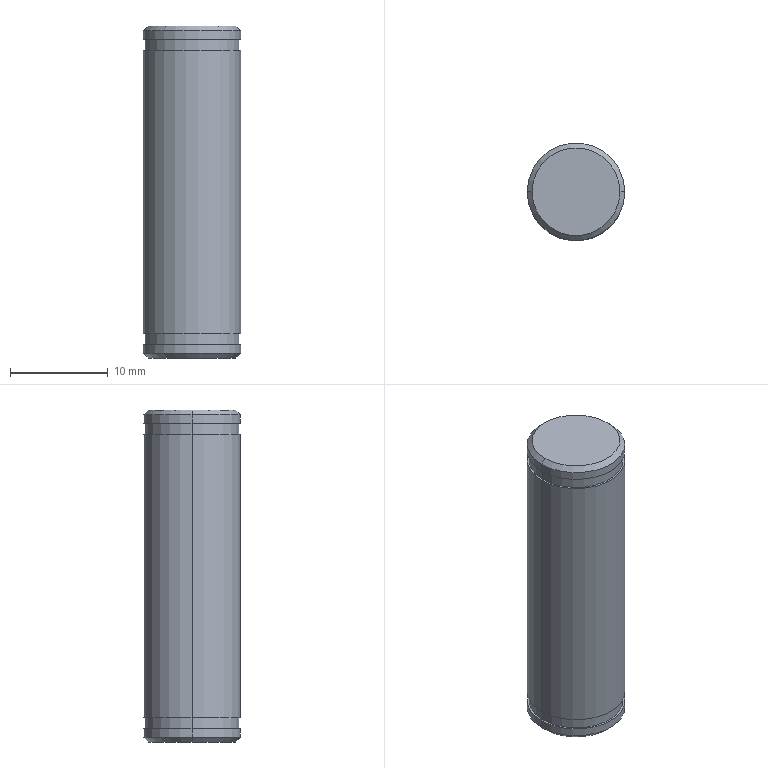Part | STEP file | CD_S03_CD-S03 | 1 solid | 20 faces | box 10 x 10 x 34 mm | volume 2649 mm3 | cylinder 10 | plane 6 | cone 4 | commonest cylinder face diameters 10 x6 9.6 x4
STEP:
#1=CARTESIAN_POINT('',(4.5,0.,-34.));
#2=VERTEX_POINT('',#1);
#3=CARTESIAN_POINT('',(-4.5,0.,-34.));
#4=VERTEX_POINT('',#3);
#5=CARTESIAN_POINT('',(0.,0.,-34.));
#6=DIRECTION('',(0.,0.,1.));
#7=DIRECTION('',(1.,0.,0.));
#8=AXIS2_PLACEMENT_3D('',#5,#6,#7);
#9=CIRCLE('',#8,4.5);
#10=EDGE_CURVE('',#2,#4,#9,.T.);
#11=ORIENTED_EDGE('',*,*,#10,.T.);
#12=CARTESIAN_POINT('',(-5.,0.,-33.5));
#13=VERTEX_POINT('',#12);
#14=CARTESIAN_POINT('',(-4.5,0.,-34.));
#15=DIRECTION('',(-0.7071,0.,0.7071));
#16=VECTOR('',#15,1000.);
#17=LINE('',#14,#16);
#18=EDGE_CURVE('',#4,#13,#17,.T.);
#19=ORIENTED_EDGE('',*,*,#18,.T.);
#20=CARTESIAN_POINT('',(5.,0.,-33.5));
#21=VERTEX_POINT('',#20);
#22=CARTESIAN_POINT('',(0.,0.,-33.5));
#23=DIRECTION('',(0.,0.,1.));
#24=DIRECTION('',(1.,0.,0.));
#25=AXIS2_PLACEMENT_3D('',#22,#23,#24);
#26=CIRCLE('',#25,5.);
#27=EDGE_CURVE('',#21,#13,#26,.T.);
#28=ORIENTED_EDGE('',*,*,#27,.F.);
#29=CARTESIAN_POINT('',(4.5,0.,-34.));
#30=DIRECTION('',(0.7071,0.,0.7071));
#31=VECTOR('',#30,1000.);
#32=LINE('',#29,#31);
#33=EDGE_CURVE('',#2,#21,#32,.T.);
#34=ORIENTED_EDGE('',*,*,#33,.F.);
#35=EDGE_LOOP('',(#11,#19,#28,#34));
#36=FACE_OUTER_BOUND('',#35,.T.);
#37=CARTESIAN_POINT('',(0.,0.,-34.));
#38=DIRECTION('',(0.,0.,1.));
#39=DIRECTION('',(1.,0.,0.));
#40=AXIS2_PLACEMENT_3D('',#37,#38,#39);
#41=CONICAL_SURFACE('',#40,4.5,0.7854);
#42=ADVANCED_FACE('',(#36),#41,.T.);
#43=ORIENTED_EDGE('',*,*,#27,.T.);
#44=CARTESIAN_POINT('',(-5.,0.,-32.65));
#45=VERTEX_POINT('',#44);
#46=CARTESIAN_POINT('',(-5.,0.,-34.));
#47=DIRECTION('',(0.,0.,1.));
#48=VECTOR('',#47,1000.);
#49=LINE('',#46,#48);
#50=EDGE_CURVE('',#13,#45,#49,.T.);
#51=ORIENTED_EDGE('',*,*,#50,.T.);
#52=CARTESIAN_POINT('',(5.,0.,-32.65));
#53=VERTEX_POINT('',#52);
#54=CARTESIAN_POINT('',(0.,0.,-32.65));
#55=DIRECTION('',(0.,0.,1.));
#56=DIRECTION('',(1.,0.,0.));
#57=AXIS2_PLACEMENT_3D('',#54,#55,#56);
#58=CIRCLE('',#57,5.);
#59=EDGE_CURVE('',#53,#45,#58,.T.);
#60=ORIENTED_EDGE('',*,*,#59,.F.);
#61=CARTESIAN_POINT('',(5.,0.,-34.));
#62=DIRECTION('',(0.,0.,1.));
#63=VECTOR('',#62,1000.);
#64=LINE('',#61,#63);
#65=EDGE_CURVE('',#21,#53,#64,.T.);
#66=ORIENTED_EDGE('',*,*,#65,.F.);
#67=EDGE_LOOP('',(#43,#51,#60,#66));
#68=FACE_OUTER_BOUND('',#67,.T.);
#69=CARTESIAN_POINT('',(0.,0.,-34.));
#70=DIRECTION('',(0.,0.,1.));
#71=DIRECTION('',(1.,0.,0.));
#72=AXIS2_PLACEMENT_3D('',#69,#70,#71);
#73=CYLINDRICAL_SURFACE('',#72,5.);
#74=ADVANCED_FACE('',(#68),#73,.T.);
#75=CARTESIAN_POINT('',(4.8,0.,-32.65));
#76=VERTEX_POINT('',#75);
#77=CARTESIAN_POINT('',(-4.8,0.,-32.65));
#78=VERTEX_POINT('',#77);
#79=CARTESIAN_POINT('',(0.,0.,-32.65));
#80=DIRECTION('',(0.,0.,1.));
#81=DIRECTION('',(1.,0.,0.));
#82=AXIS2_PLACEMENT_3D('',#79,#80,#81);
#83=CIRCLE('',#82,4.8);
#84=EDGE_CURVE('',#76,#78,#83,.T.);
#85=ORIENTED_EDGE('',*,*,#84,.T.);
#86=CARTESIAN_POINT('',(-4.8,0.,-31.5));
#87=VERTEX_POINT('',#86);
#88=CARTESIAN_POINT('',(-4.8,0.,-34.));
#89=DIRECTION('',(0.,0.,1.));
#90=VECTOR('',#89,1000.);
#91=LINE('',#88,#90);
#92=EDGE_CURVE('',#78,#87,#91,.T.);
#93=ORIENTED_EDGE('',*,*,#92,.T.);
#94=CARTESIAN_POINT('',(4.8,0.,-31.5));
#95=VERTEX_POINT('',#94);
#96=CARTESIAN_POINT('',(0.,0.,-31.5));
#97=DIRECTION('',(0.,0.,1.));
#98=DIRECTION('',(1.,0.,0.));
#99=AXIS2_PLACEMENT_3D('',#96,#97,#98);
#100=CIRCLE('',#99,4.8);
#101=EDGE_CURVE('',#95,#87,#100,.T.);
#102=ORIENTED_EDGE('',*,*,#101,.F.);
#103=CARTESIAN_POINT('',(4.8,0.,-34.));
#104=DIRECTION('',(0.,0.,1.));
#105=VECTOR('',#104,1000.);
#106=LINE('',#103,#105);
#107=EDGE_CURVE('',#76,#95,#106,.T.);
#108=ORIENTED_EDGE('',*,*,#107,.F.);
#109=EDGE_LOOP('',(#85,#93,#102,#108));
#110=FACE_OUTER_BOUND('',#109,.T.);
#111=CARTESIAN_POINT('',(0.,0.,-34.));
#112=DIRECTION('',(0.,0.,1.));
#113=DIRECTION('',(1.,0.,0.));
#114=AXIS2_PLACEMENT_3D('',#111,#112,#113);
#115=CYLINDRICAL_SURFACE('',#114,4.8);
#116=ADVANCED_FACE('',(#110),#115,.T.);
#117=CARTESIAN_POINT('',(5.,0.,-31.5));
#118=VERTEX_POINT('',#117);
#119=CARTESIAN_POINT('',(-5.,0.,-31.5));
#120=VERTEX_POINT('',#119);
#121=CARTESIAN_POINT('',(0.,0.,-31.5));
#122=DIRECTION('',(0.,0.,1.));
#123=DIRECTION('',(1.,0.,0.));
#124=AXIS2_PLACEMENT_3D('',#121,#122,#123);
#125=CIRCLE('',#124,5.);
#126=EDGE_CURVE('',#118,#120,#125,.T.);
#127=ORIENTED_EDGE('',*,*,#126,.T.);
#128=CARTESIAN_POINT('',(-5.,0.,-2.5));
#129=VERTEX_POINT('',#128);
#130=CARTESIAN_POINT('',(-5.,0.,-34.));
#131=DIRECTION('',(0.,0.,1.));
#132=VECTOR('',#131,1000.);
#133=LINE('',#130,#132);
#134=EDGE_CURVE('',#120,#129,#133,.T.);
#135=ORIENTED_EDGE('',*,*,#134,.T.);
#136=CARTESIAN_POINT('',(5.,0.,-2.5));
#137=VERTEX_POINT('',#136);
#138=CARTESIAN_POINT('',(0.,0.,-2.5));
#139=DIRECTION('',(0.,0.,1.));
#140=DIRECTION('',(1.,0.,0.));
#141=AXIS2_PLACEMENT_3D('',#138,#139,#140);
#142=CIRCLE('',#141,5.);
#143=EDGE_CURVE('',#137,#129,#142,.T.);
#144=ORIENTED_EDGE('',*,*,#143,.F.);
#145=CARTESIAN_POINT('',(5.,0.,-34.));
#146=DIRECTION('',(0.,0.,1.));
#147=VECTOR('',#146,1000.);
#148=LINE('',#145,#147);
#149=EDGE_CURVE('',#118,#137,#148,.T.);
#150=ORIENTED_EDGE('',*,*,#149,.F.);
#151=EDGE_LOOP('',(#127,#135,#144,#150));
#152=FACE_OUTER_BOUND('',#151,.T.);
#153=CARTESIAN_POINT('',(0.,0.,-34.));
#154=DIRECTION('',(0.,0.,1.));
#155=DIRECTION('',(1.,0.,0.));
#156=AXIS2_PLACEMENT_3D('',#153,#154,#155);
#157=CYLINDRICAL_SURFACE('',#156,5.);
#158=ADVANCED_FACE('',(#152),#157,.T.);
#159=CARTESIAN_POINT('',(4.8,0.,-2.5));
#160=VERTEX_POINT('',#159);
#161=CARTESIAN_POINT('',(-4.8,0.,-2.5));
#162=VERTEX_POINT('',#161);
#163=CARTESIAN_POINT('',(0.,0.,-2.5));
#164=DIRECTION('',(0.,0.,1.));
#165=DIRECTION('',(1.,0.,0.));
#166=AXIS2_PLACEMENT_3D('',#163,#164,#165);
#167=CIRCLE('',#166,4.8);
#168=EDGE_CURVE('',#160,#162,#167,.T.);
#169=ORIENTED_EDGE('',*,*,#168,.T.);
#170=CARTESIAN_POINT('',(-4.8,0.,-1.35));
#171=VERTEX_POINT('',#170);
#172=CARTESIAN_POINT('',(-4.8,0.,-34.));
#173=DIRECTION('',(0.,0.,1.));
#174=VECTOR('',#173,1000.);
#175=LINE('',#172,#174);
#176=EDGE_CURVE('',#162,#171,#175,.T.);
#177=ORIENTED_EDGE('',*,*,#176,.T.);
#178=CARTESIAN_POINT('',(4.8,0.,-1.35));
#179=VERTEX_POINT('',#178);
#180=CARTESIAN_POINT('',(0.,0.,-1.35));
#181=DIRECTION('',(0.,0.,1.));
#182=DIRECTION('',(1.,0.,0.));
#183=AXIS2_PLACEMENT_3D('',#180,#181,#182);
#184=CIRCLE('',#183,4.8);
#185=EDGE_CURVE('',#179,#171,#184,.T.);
#186=ORIENTED_EDGE('',*,*,#185,.F.);
#187=CARTESIAN_POINT('',(4.8,0.,-34.));
#188=DIRECTION('',(0.,0.,1.));
#189=VECTOR('',#188,1000.);
#190=LINE('',#187,#189);
#191=EDGE_CURVE('',#160,#179,#190,.T.);
#192=ORIENTED_EDGE('',*,*,#191,.F.);
#193=EDGE_LOOP('',(#169,#177,#186,#192));
#194=FACE_OUTER_BOUND('',#193,.T.);
#195=CARTESIAN_POINT('',(0.,0.,-34.));
#196=DIRECTION('',(0.,0.,1.));
#197=DIRECTION('',(1.,0.,0.));
#198=AXIS2_PLACEMENT_3D('',#195,#196,#197);
#199=CYLINDRICAL_SURFACE('',#198,4.8);
#200=ADVANCED_FACE('',(#194),#199,.T.);
#201=CARTESIAN_POINT('',(5.,0.,-1.35));
#202=VERTEX_POINT('',#201);
#203=CARTESIAN_POINT('',(-5.,0.,-1.35));
#204=VERTEX_POINT('',#203);
#205=CARTESIAN_POINT('',(0.,0.,-1.35));
#206=DIRECTION('',(0.,0.,1.));
#207=DIRECTION('',(1.,0.,0.));
#208=AXIS2_PLACEMENT_3D('',#205,#206,#207);
#209=CIRCLE('',#208,5.);
#210=EDGE_CURVE('',#202,#204,#209,.T.);
#211=ORIENTED_EDGE('',*,*,#210,.T.);
#212=CARTESIAN_POINT('',(-5.,0.,-0.5));
#213=VERTEX_POINT('',#212);
#214=CARTESIAN_POINT('',(-5.,0.,-34.));
#215=DIRECTION('',(0.,0.,1.));
#216=VECTOR('',#215,1000.);
#217=LINE('',#214,#216);
#218=EDGE_CURVE('',#204,#213,#217,.T.);
#219=ORIENTED_EDGE('',*,*,#218,.T.);
#220=CARTESIAN_POINT('',(5.,0.,-0.5));
#221=VERTEX_POINT('',#220);
#222=CARTESIAN_POINT('',(0.,0.,-0.5));
#223=DIRECTION('',(0.,0.,1.));
#224=DIRECTION('',(1.,0.,0.));
#225=AXIS2_PLACEMENT_3D('',#222,#223,#224);
#226=CIRCLE('',#225,5.);
#227=EDGE_CURVE('',#221,#213,#226,.T.);
#228=ORIENTED_EDGE('',*,*,#227,.F.);
#229=CARTESIAN_POINT('',(5.,0.,-34.));
#230=DIRECTION('',(0.,0.,1.));
#231=VECTOR('',#230,1000.);
#232=LINE('',#229,#231);
#233=EDGE_CURVE('',#202,#221,#232,.T.);
#234=ORIENTED_EDGE('',*,*,#233,.F.);
#235=EDGE_LOOP('',(#211,#219,#228,#234));
#236=FACE_OUTER_BOUND('',#235,.T.);
#237=CARTESIAN_POINT('',(0.,0.,-34.));
#238=DIRECTION('',(0.,0.,1.));
#239=DIRECTION('',(1.,0.,0.));
#240=AXIS2_PLACEMENT_3D('',#237,#238,#239);
#241=CYLINDRICAL_SURFACE('',#240,5.);
#242=ADVANCED_FACE('',(#236),#241,.T.);
#243=CARTESIAN_POINT('',(4.5,0.,0.));
#244=VERTEX_POINT('',#243);
#245=CARTESIAN_POINT('',(-4.5,0.,0.));
#246=VERTEX_POINT('',#245);
#247=CARTESIAN_POINT('',(0.,0.,0.));
#248=DIRECTION('',(0.,0.,1.));
#249=DIRECTION('',(1.,0.,0.));
#250=AXIS2_PLACEMENT_3D('',#247,#248,#249);
#251=CIRCLE('',#250,4.5);
#252=EDGE_CURVE('',#244,#246,#251,.T.);
#253=ORIENTED_EDGE('',*,*,#252,.F.);
#254=CARTESIAN_POINT('',(5.,0.,-0.5));
#255=DIRECTION('',(0.7071,0.,-0.7071));
#256=VECTOR('',#255,1000.);
#257=LINE('',#254,#256);
#258=EDGE_CURVE('',#244,#221,#257,.T.);
#259=ORIENTED_EDGE('',*,*,#258,.T.);
#260=ORIENTED_EDGE('',*,*,#227,.T.);
#261=CARTESIAN_POINT('',(-5.,0.,-0.5));
#262=DIRECTION('',(-0.7071,0.,-0.7071));
#263=VECTOR('',#262,1000.);
#264=LINE('',#261,#263);
#265=EDGE_CURVE('',#246,#213,#264,.T.);
#266=ORIENTED_EDGE('',*,*,#265,.F.);
#267=EDGE_LOOP('',(#253,#259,#260,#266));
#268=FACE_OUTER_BOUND('',#267,.T.);
#269=CARTESIAN_POINT('',(0.,0.,-0.5));
#270=DIRECTION('',(0.,0.,-1.));
#271=DIRECTION('',(-1.,0.,0.));
#272=AXIS2_PLACEMENT_3D('',#269,#270,#271);
#273=CONICAL_SURFACE('',#272,5.,0.7854);
#274=ADVANCED_FACE('',(#268),#273,.T.);
#275=CARTESIAN_POINT('',(0.,0.,0.));
#276=DIRECTION('',(0.,0.,1.));
#277=DIRECTION('',(1.,0.,0.));
#278=AXIS2_PLACEMENT_3D('',#275,#276,#277);
#279=CIRCLE('',#278,4.5);
#280=EDGE_CURVE('',#246,#244,#279,.T.);
#281=ORIENTED_EDGE('',*,*,#280,.T.);
#282=ORIENTED_EDGE('',*,*,#252,.T.);
#283=EDGE_LOOP('',(#281,#282));
#284=FACE_OUTER_BOUND('',#283,.T.);
#285=CARTESIAN_POINT('',(0.,0.,0.));
#286=DIRECTION('',(0.,0.,-1.));
#287=DIRECTION('',(-1.,0.,0.));
#288=AXIS2_PLACEMENT_3D('',#285,#286,#287);
#289=PLANE('',#288);
#290=ADVANCED_FACE('',(#284),#289,.F.);
#291=ORIENTED_EDGE('',*,*,#258,.F.);
#292=ORIENTED_EDGE('',*,*,#280,.F.);
#293=ORIENTED_EDGE('',*,*,#265,.T.);
#294=CARTESIAN_POINT('',(0.,0.,-0.5));
#295=DIRECTION('',(0.,0.,1.));
#296=DIRECTION('',(1.,0.,0.));
#297=AXIS2_PLACEMENT_3D('',#294,#295,#296);
#298=CIRCLE('',#297,5.);
#299=EDGE_CURVE('',#213,#221,#298,.T.);
#300=ORIENTED_EDGE('',*,*,#299,.T.);
#301=EDGE_LOOP('',(#291,#292,#293,#300));
#302=FACE_OUTER_BOUND('',#301,.T.);
#303=CARTESIAN_POINT('',(0.,0.,-0.5));
#304=DIRECTION('',(0.,0.,-1.));
#305=DIRECTION('',(-1.,0.,0.));
#306=AXIS2_PLACEMENT_3D('',#303,#304,#305);
#307=CONICAL_SURFACE('',#306,5.,0.7854);
#308=ADVANCED_FACE('',(#302),#307,.T.);
#309=ORIENTED_EDGE('',*,*,#218,.F.);
#310=CARTESIAN_POINT('',(0.,0.,-1.35));
#311=DIRECTION('',(0.,0.,1.));
#312=DIRECTION('',(1.,0.,0.));
#313=AXIS2_PLACEMENT_3D('',#310,#311,#312);
#314=CIRCLE('',#313,5.);
#315=EDGE_CURVE('',#204,#202,#314,.T.);
#316=ORIENTED_EDGE('',*,*,#315,.T.);
#317=ORIENTED_EDGE('',*,*,#233,.T.);
#318=ORIENTED_EDGE('',*,*,#299,.F.);
#319=EDGE_LOOP('',(#309,#316,#317,#318));
#320=FACE_OUTER_BOUND('',#319,.T.);
#321=CARTESIAN_POINT('',(0.,0.,-34.));
#322=DIRECTION('',(0.,0.,1.));
#323=DIRECTION('',(1.,0.,0.));
#324=AXIS2_PLACEMENT_3D('',#321,#322,#323);
#325=CYLINDRICAL_SURFACE('',#324,5.);
#326=ADVANCED_FACE('',(#320),#325,.T.);
#327=ORIENTED_EDGE('',*,*,#210,.F.);
#328=ORIENTED_EDGE('',*,*,#315,.F.);
#329=EDGE_LOOP('',(#327,#328));
#330=FACE_OUTER_BOUND('',#329,.T.);
#331=ORIENTED_EDGE('',*,*,#185,.T.);
#332=CARTESIAN_POINT('',(0.,0.,-1.35));
#333=DIRECTION('',(0.,0.,1.));
#334=DIRECTION('',(1.,0.,0.));
#335=AXIS2_PLACEMENT_3D('',#332,#333,#334);
#336=CIRCLE('',#335,4.8);
#337=EDGE_CURVE('',#171,#179,#336,.T.);
#338=ORIENTED_EDGE('',*,*,#337,.T.);
#339=EDGE_LOOP('',(#331,#338));
#340=FACE_BOUND('',#339,.T.);
#341=CARTESIAN_POINT('',(0.,5.,-1.35));
#342=DIRECTION('',(0.,0.,1.));
#343=DIRECTION('',(1.,0.,0.));
#344=AXIS2_PLACEMENT_3D('',#341,#342,#343);
#345=PLANE('',#344);
#346=ADVANCED_FACE('',(#330,#340),#345,.F.);
#347=ORIENTED_EDGE('',*,*,#176,.F.);
#348=CARTESIAN_POINT('',(0.,0.,-2.5));
#349=DIRECTION('',(0.,0.,1.));
#350=DIRECTION('',(1.,0.,0.));
#351=AXIS2_PLACEMENT_3D('',#348,#349,#350);
#352=CIRCLE('',#351,4.8);
#353=EDGE_CURVE('',#162,#160,#352,.T.);
#354=ORIENTED_EDGE('',*,*,#353,.T.);
#355=ORIENTED_EDGE('',*,*,#191,.T.);
#356=ORIENTED_EDGE('',*,*,#337,.F.);
#357=EDGE_LOOP('',(#347,#354,#355,#356));
#358=FACE_OUTER_BOUND('',#357,.T.);
#359=CARTESIAN_POINT('',(0.,0.,-34.));
#360=DIRECTION('',(0.,0.,1.));
#361=DIRECTION('',(1.,0.,0.));
#362=AXIS2_PLACEMENT_3D('',#359,#360,#361);
#363=CYLINDRICAL_SURFACE('',#362,4.8);
#364=ADVANCED_FACE('',(#358),#363,.T.);
#365=ORIENTED_EDGE('',*,*,#168,.F.);
#366=ORIENTED_EDGE('',*,*,#353,.F.);
#367=EDGE_LOOP('',(#365,#366));
#368=FACE_BOUND('',#367,.T.);
#369=ORIENTED_EDGE('',*,*,#143,.T.);
#370=CARTESIAN_POINT('',(0.,0.,-2.5));
#371=DIRECTION('',(0.,0.,1.));
#372=DIRECTION('',(1.,0.,0.));
#373=AXIS2_PLACEMENT_3D('',#370,#371,#372);
#374=CIRCLE('',#373,5.);
#375=EDGE_CURVE('',#129,#137,#374,.T.);
#376=ORIENTED_EDGE('',*,*,#375,.T.);
#377=EDGE_LOOP('',(#369,#376));
#378=FACE_OUTER_BOUND('',#377,.T.);
#379=CARTESIAN_POINT('',(0.,4.8,-2.5));
#380=DIRECTION('',(0.,0.,-1.));
#381=DIRECTION('',(-1.,0.,0.));
#382=AXIS2_PLACEMENT_3D('',#379,#380,#381);
#383=PLANE('',#382);
#384=ADVANCED_FACE('',(#368,#378),#383,.F.);
#385=ORIENTED_EDGE('',*,*,#134,.F.);
#386=CARTESIAN_POINT('',(0.,0.,-31.5));
#387=DIRECTION('',(0.,0.,1.));
#388=DIRECTION('',(1.,0.,0.));
#389=AXIS2_PLACEMENT_3D('',#386,#387,#388);
#390=CIRCLE('',#389,5.);
#391=EDGE_CURVE('',#120,#118,#390,.T.);
#392=ORIENTED_EDGE('',*,*,#391,.T.);
#393=ORIENTED_EDGE('',*,*,#149,.T.);
#394=ORIENTED_EDGE('',*,*,#375,.F.);
#395=EDGE_LOOP('',(#385,#392,#393,#394));
#396=FACE_OUTER_BOUND('',#395,.T.);
#397=CARTESIAN_POINT('',(0.,0.,-34.));
#398=DIRECTION('',(0.,0.,1.));
#399=DIRECTION('',(1.,0.,0.));
#400=AXIS2_PLACEMENT_3D('',#397,#398,#399);
#401=CYLINDRICAL_SURFACE('',#400,5.);
#402=ADVANCED_FACE('',(#396),#401,.T.);
#403=ORIENTED_EDGE('',*,*,#126,.F.);
#404=ORIENTED_EDGE('',*,*,#391,.F.);
#405=EDGE_LOOP('',(#403,#404));
#406=FACE_OUTER_BOUND('',#405,.T.);
#407=ORIENTED_EDGE('',*,*,#101,.T.);
#408=CARTESIAN_POINT('',(0.,0.,-31.5));
#409=DIRECTION('',(0.,0.,1.));
#410=DIRECTION('',(1.,0.,0.));
#411=AXIS2_PLACEMENT_3D('',#408,#409,#410);
#412=CIRCLE('',#411,4.8);
#413=EDGE_CURVE('',#87,#95,#412,.T.);
#414=ORIENTED_EDGE('',*,*,#413,.T.);
#415=EDGE_LOOP('',(#407,#414));
#416=FACE_BOUND('',#415,.T.);
#417=CARTESIAN_POINT('',(0.,5.,-31.5));
#418=DIRECTION('',(0.,0.,1.));
#419=DIRECTION('',(1.,0.,0.));
#420=AXIS2_PLACEMENT_3D('',#417,#418,#419);
#421=PLANE('',#420);
#422=ADVANCED_FACE('',(#406,#416),#421,.F.);
#423=ORIENTED_EDGE('',*,*,#92,.F.);
#424=CARTESIAN_POINT('',(0.,0.,-32.65));
#425=DIRECTION('',(0.,0.,1.));
#426=DIRECTION('',(1.,0.,0.));
#427=AXIS2_PLACEMENT_3D('',#424,#425,#426);
#428=CIRCLE('',#427,4.8);
#429=EDGE_CURVE('',#78,#76,#428,.T.);
#430=ORIENTED_EDGE('',*,*,#429,.T.);
#431=ORIENTED_EDGE('',*,*,#107,.T.);
#432=ORIENTED_EDGE('',*,*,#413,.F.);
#433=EDGE_LOOP('',(#423,#430,#431,#432));
#434=FACE_OUTER_BOUND('',#433,.T.);
#435=CARTESIAN_POINT('',(0.,0.,-34.));
#436=DIRECTION('',(0.,0.,1.));
#437=DIRECTION('',(1.,0.,0.));
#438=AXIS2_PLACEMENT_3D('',#435,#436,#437);
#439=CYLINDRICAL_SURFACE('',#438,4.8);
#440=ADVANCED_FACE('',(#434),#439,.T.);
#441=ORIENTED_EDGE('',*,*,#84,.F.);
#442=ORIENTED_EDGE('',*,*,#429,.F.);
#443=EDGE_LOOP('',(#441,#442));
#444=FACE_BOUND('',#443,.T.);
#445=ORIENTED_EDGE('',*,*,#59,.T.);
#446=CARTESIAN_POINT('',(0.,0.,-32.65));
#447=DIRECTION('',(0.,0.,1.));
#448=DIRECTION('',(1.,0.,0.));
#449=AXIS2_PLACEMENT_3D('',#446,#447,#448);
#450=CIRCLE('',#449,5.);
#451=EDGE_CURVE('',#45,#53,#450,.T.);
#452=ORIENTED_EDGE('',*,*,#451,.T.);
#453=EDGE_LOOP('',(#445,#452));
#454=FACE_OUTER_BOUND('',#453,.T.);
#455=CARTESIAN_POINT('',(0.,4.8,-32.65));
#456=DIRECTION('',(0.,0.,-1.));
#457=DIRECTION('',(-1.,0.,0.));
#458=AXIS2_PLACEMENT_3D('',#455,#456,#457);
#459=PLANE('',#458);
#460=ADVANCED_FACE('',(#444,#454),#459,.F.);
#461=ORIENTED_EDGE('',*,*,#50,.F.);
#462=CARTESIAN_POINT('',(0.,0.,-33.5));
#463=DIRECTION('',(0.,0.,1.));
#464=DIRECTION('',(1.,0.,0.));
#465=AXIS2_PLACEMENT_3D('',#462,#463,#464);
#466=CIRCLE('',#465,5.);
#467=EDGE_CURVE('',#13,#21,#466,.T.);
#468=ORIENTED_EDGE('',*,*,#467,.T.);
#469=ORIENTED_EDGE('',*,*,#65,.T.);
#470=ORIENTED_EDGE('',*,*,#451,.F.);
#471=EDGE_LOOP('',(#461,#468,#469,#470));
#472=FACE_OUTER_BOUND('',#471,.T.);
#473=CARTESIAN_POINT('',(0.,0.,-34.));
#474=DIRECTION('',(0.,0.,1.));
#475=DIRECTION('',(1.,0.,0.));
#476=AXIS2_PLACEMENT_3D('',#473,#474,#475);
#477=CYLINDRICAL_SURFACE('',#476,5.);
#478=ADVANCED_FACE('',(#472),#477,.T.);
#479=ORIENTED_EDGE('',*,*,#18,.F.);
#480=CARTESIAN_POINT('',(0.,0.,-34.));
#481=DIRECTION('',(0.,0.,1.));
#482=DIRECTION('',(1.,0.,0.));
#483=AXIS2_PLACEMENT_3D('',#480,#481,#482);
#484=CIRCLE('',#483,4.5);
#485=EDGE_CURVE('',#4,#2,#484,.T.);
#486=ORIENTED_EDGE('',*,*,#485,.T.);
#487=ORIENTED_EDGE('',*,*,#33,.T.);
#488=ORIENTED_EDGE('',*,*,#467,.F.);
#489=EDGE_LOOP('',(#479,#486,#487,#488));
#490=FACE_OUTER_BOUND('',#489,.T.);
#491=CARTESIAN_POINT('',(0.,0.,-34.));
#492=DIRECTION('',(0.,0.,1.));
#493=DIRECTION('',(1.,0.,0.));
#494=AXIS2_PLACEMENT_3D('',#491,#492,#493);
#495=CONICAL_SURFACE('',#494,4.5,0.7854);
#496=ADVANCED_FACE('',(#490),#495,.T.);
#497=ORIENTED_EDGE('',*,*,#10,.F.);
#498=ORIENTED_EDGE('',*,*,#485,.F.);
#499=EDGE_LOOP('',(#497,#498));
#500=FACE_OUTER_BOUND('',#499,.T.);
#501=CARTESIAN_POINT('',(0.,4.5,-34.));
#502=DIRECTION('',(0.,0.,1.));
#503=DIRECTION('',(1.,0.,0.));
#504=AXIS2_PLACEMENT_3D('',#501,#502,#503);
#505=PLANE('',#504);
#506=ADVANCED_FACE('',(#500),#505,.F.);
#507=CLOSED_SHELL('',(#42,#74,#116,#158,#200,#242,#274,#290,#308,#326,#346,#364,#384,#402,#422,#440,#460,#478,#496,#506));
#508=MANIFOLD_SOLID_BREP('',#507);
#509=CARTESIAN_POINT('',(0.,0.,0.));
#510=DIRECTION('',(0.,0.,1.));
#511=DIRECTION('',(1.,0.,0.));
#512=AXIS2_PLACEMENT_3D('',#509,#510,#511);
#513=(LENGTH_UNIT()NAMED_UNIT(*)SI_UNIT(.MILLI.,.METRE.));
#514=UNCERTAINTY_MEASURE_WITH_UNIT(LENGTH_MEASURE(0.00001),#513,'','');
#515=(NAMED_UNIT(*)PLANE_ANGLE_UNIT()SI_UNIT($,.RADIAN.));
#516=(NAMED_UNIT(*)SI_UNIT($,.STERADIAN.)SOLID_ANGLE_UNIT());
#517=(GEOMETRIC_REPRESENTATION_CONTEXT(3)GLOBAL_UNCERTAINTY_ASSIGNED_CONTEXT((#514))GLOBAL_UNIT_ASSIGNED_CONTEXT((#513,#515,#516))REPRESENTATION_CONTEXT('',''));
#518=ADVANCED_BREP_SHAPE_REPRESENTATION('',(#508,#512),#517);